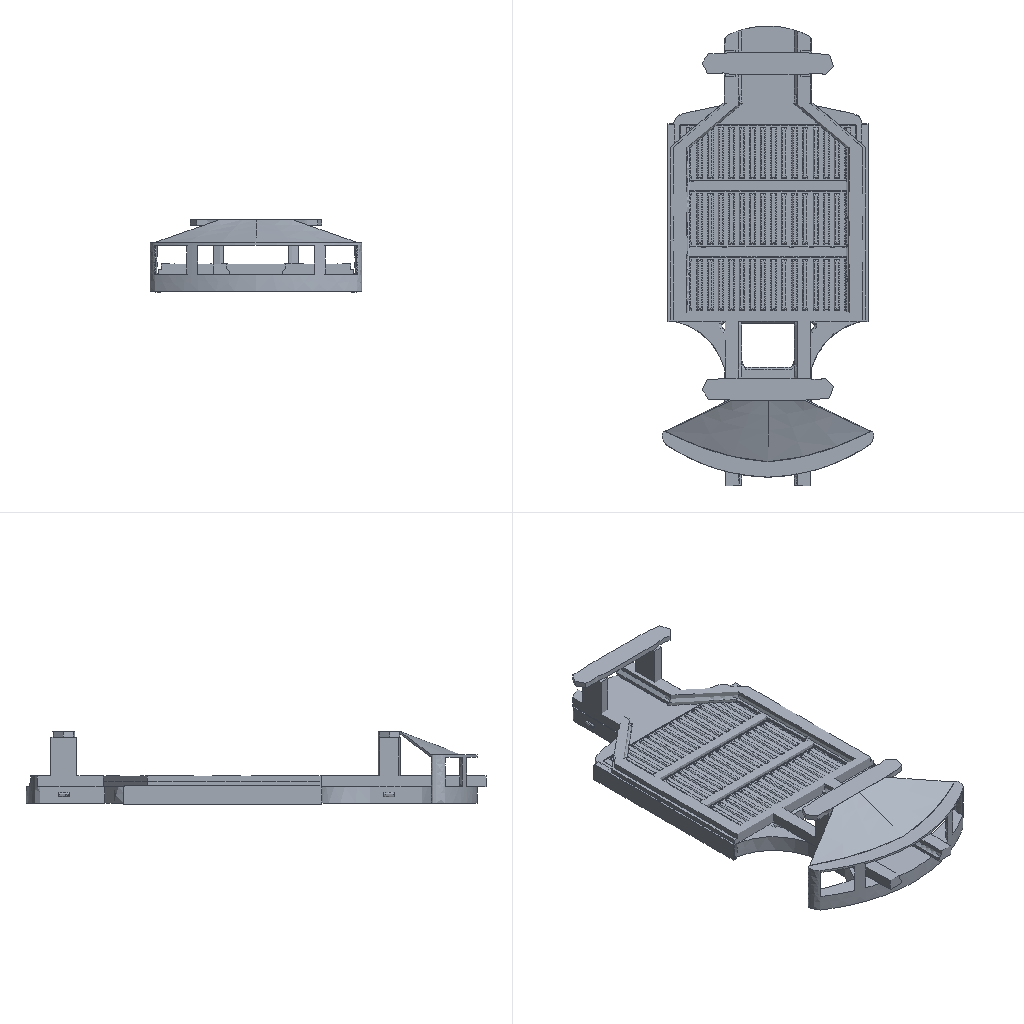Simulation study | ansys workbench
Ansys APDL input file, long lists of numbers shortened:
/batch
/config,noeldb,1     ! force off writing results to database
*get,_wallstrt,active,,time,wall
! ANSYS input file written by Workbench version 2022 R1
! File used for geometry attach: F:\ansys（分析文件汇总)\底盘有限元分析\ansys\dipan.STEP
/title,wbnew--____ (C5)
! ****** Begin Custom Load Command Snippet ******
/COM, ACT Extensions:
/COM,     LSDYNA, 2021.1
/COM,
! ****** End   Custom Load Command Snippet ******
*DIM,_wb_ProjectScratch_dir,string,248
_wb_ProjectScratch_dir(1) = 'C:\Users\Administrator\AppData\Local\Temp\WB_Administrator_26060_2\_ProjectScratch\Scr306D\'
*DIM,_wb_SolverFiles_dir,string,248
_wb_SolverFiles_dir(1) = 'C:\Users\Administrator\AppData\Local\Temp\WB_Administrator_26060_2\wbnew_files\dp0\SYS-1\MECH\'
*DIM,_wb_userfiles_dir,string,248
_wb_userfiles_dir(1) = 'C:\Users\Administrator\AppData\Local\Temp\WB_Administrator_26060_2\wbnew_files\user_files\'
/com,--- Data in consistent NMM units. See Solving Units in the help system for more information.
/units,MPA
/nopr
/wb,file,start              !  signify a WB generated input file
/prep7
! Turn off shape checking because checks already performed inside WB mesher.
! See help system for more information.
SHPP,OFF,,NOWARN
/nolist
etcon,set             ! allow ANSYS to choose best KEYOP's for 180x elements, resets any applicable keyopt to MAPDL defaults
/com,*********** Nodes for the whole assembly ***********
nblock,3,,302792
(1i9,3e20.9e3)
        1     2.552000817E+02    -4.340854422E+02     3.633624358E+02
! (275265 more lines like these left out)
-1
/wb,elem,start            !  set before creation of elements
/com,*********** Elements for Body 1 "dipan-FreeParts|NONE" ***********
et,1,187
eblock,19,solid,,173485
(19i9)
        1        1        1        1        0        0        0        0       10        0       19    13623    39379    40222    40211   140088   275016   140091   140090
! (346969 more lines like these left out)
-1
/com,*********** Elements for Body 2 "dipan-FreeParts|NONE[2]" ***********
et,2,186
keyo,2,2,1          ! set full integration on SOLID186
eblock,19,solid,,9
(19i9)
        2        2        2        2        0        0        0        0       20        0        1        4       21       24       25        5       19       20       16
! (17 more lines like these left out)
-1
/com,*********** Elements for Body 3 "dipan-FreeParts|NONE[3]" ***********
et,3,186
keyo,3,2,1          ! set full integration on SOLID186
eblock,19,solid,,9
(19i9)
        3        3        3        3        0        0        0        0       20        0       10      100      117      120      121      101      115      116      112
! (17 more lines like these left out)
-1
/wb,elem,end               !  done creating elements
/com,*********** Send User Defined Coordinate System(s) ***********
csys,0
toffst,273.15,  ! Temperature offset from absolute zero
/com,*********** Set Reference Temperature ***********
tref,22.
/wb,mat,start              !  starting to send materials
/com,*********** Send Materials ***********
Temperature = 'TEMP' ! Temperature
MP,DENS,1,7.85e-09,	! tonne mm^-3
MP,ALPX,1,1.2e-05,	! C^-1
MP,C,1,434000000,	! mm^2 s^-2 C^-1
MP,KXX,1,60.5,	! tonne mm s^-3 C^-1
MP,RSVX,1,0.00017,	! ohm mm
MP,EX,1,200000,	! tonne s^-2 mm^-1
MP,NUXY,1,0.3,
MP,MURX,1,10000,
Temperature = 'TEMP' ! Temperature
MP,DENS,2,7.85e-09,	! tonne mm^-3
MP,ALPX,2,1.2e-05,	! C^-1
MP,C,2,434000000,	! mm^2 s^-2 C^-1
MP,KXX,2,60.5,	! tonne mm s^-3 C^-1
MP,RSVX,2,0.00017,	! ohm mm
MP,EX,2,200000,	! tonne s^-2 mm^-1
MP,NUXY,2,0.3,
MP,MURX,2,10000,
Temperature = 'TEMP' ! Temperature
MP,DENS,3,7.85e-09,	! tonne mm^-3
MP,ALPX,3,1.2e-05,	! C^-1
MP,C,3,434000000,	! mm^2 s^-2 C^-1
MP,KXX,3,60.5,	! tonne mm s^-3 C^-1
MP,RSVX,3,0.00017,	! ohm mm
MP,EX,3,200000,	! tonne s^-2 mm^-1
MP,NUXY,3,0.3,
MP,MURX,3,10000,
/wb,mat,end                !  done sending materials
!************************* Model Summary ********************
!dipan-FreeParts|NONE,	结构钢,	matid,	1
!dipan-FreeParts|NONE[2],	结构钢,	matid,	2
!dipan-FreeParts|NONE[3],	结构钢,	matid,	3
!************************* End Model Summary ********************
! get the diagonal of the bounding box. Needed later for other things
*get,_xmin,node,,mnloc,x
*get,_ymin,node,,mnloc,y
*get,_zmin,node,,mnloc,z
*get,_xmax,node,,mxloc,x
*get,_ymax,node,,mxloc,y
*get,_zmax,node,,mxloc,z
_ASMDIAG=(_xmax-_xmin)*(_xmax-_xmin)+(_ymax-_ymin)*(_ymax-_ymin)+(_zmax-_zmin)*(_zmax-_zmin)
_ASMDIAG=SQRT(_ASMDIAG)
/wb,contact,start          !  starting to send contact
/com,*********** Create Contact "接触区域 3" ***********
/com,            Real Constant Set For Above Contact Is 5 & 4
*set,tid,5
*set,cid,4
r,tid
r,cid
et,tid,170
et,cid,174
eblock,10,,,3
(15i9)
   216164        5        5        5        0       30       29       12       11       94       69       66       67
   216165        5        5        5        0       29       28       13       12       93       71       68       69
   216166        5        5        5        0       28       23       17       13       88       79       70       71
-1
eblock,10,,,3
(15i9)
   216167        4        4        4        0       30       29       12       11       94       69       66       67
   216168        4        4        4        0       29       28       13       12       93       71       68       69
   216169        4        4        4        0       28       23       17       13       88       79       70       71
-1
eblock,10,,,3
(15i9)
   216170        4        5        4        0      110      111      122      123      168      171      187      169
   216171        4        5        4        0      111      112      121      122      170      173      186      171
   216172        4        5        4        0      112      116      120      121      172      180      185      173
-1
eblock,10,,,3
(15i9)
   216173        5        4        5        0      110      111      122      123      168      171      187      169
   216174        5        4        5        0      111      112      121      122      170      173      186      171
   216175        5        4        5        0      112      116      120      121      172      180      185      173
-1
keyo,cid,8,2               ! auto create asymmetric contact (from Program Controlled setting)
keyo,cid,10,0              ! adjust contact stiffness each NR iteration (from Program Controlled setting)
keyo,cid,12,5              ! bonded always
keyo,cid,18,1              ! small sliding turned on by application
keyo,cid,2,0               ! augmented Lagrange (from Program Controlled setting)
keyo,cid,4,0               ! on Gauss point (from Program Controlled setting)
keyo,cid,9,1               ! ignore initial gaps/penetration
keyo,cid,7,0               ! No Prediction
rmod,tid,3,10.      ! FKN
rmod,tid,5,0.       ! ICONT
rmod,tid,6,0.       ! PINB
rmod,tid,10,0.      ! CNOF
rmod,tid,12,0.      ! FKT
rmod,tid,36,47      ! WB DSID
rmod,cid,3,10.      ! FKN
rmod,cid,5,0.       ! ICONT
rmod,cid,6,0.       ! PINB
rmod,cid,10,0.      ! CNOF
rmod,cid,12,0.      ! FKT
rmod,cid,36,47      ! WB DSID
nsel,all
esel,all
/wb,contact,end            !  done creating contacts
/golist
/wb,load,start             !  starting to send loads
/com,*********** Fixed Supports ***********
CMBLOCK,_FIXEDSU,NODE,      435
(8i10)
         5         6         7         8         9        10        11        12
! (54 more lines like these left out)
cmsel,s,_FIXEDSU
d,all,all
nsel,all
/com,*********** Define Force Using Surface Effect Elements ***********
local,12,0,0.,0.,0.,0.,0.,0.
csys,0
et,6,154
eblock,10,,,13183
(15i9)
   216176        6        6        6       12    13326    13856    13958    13958   137814   141428    13958   137816
! (13182 more lines like these left out)
-1
esel,s,type,,6
keyop,6,2,1                ! Apply load in local coordinate system
keyop,6,7,1                ! Use original area so load is constant in large deformation
esel,all
/gst,on,on
fini
*get,_numnode,node,0,count
*get,_numelem,elem,0,count
*get, _MAXELEMNUM, elem, 0, NUM, MAX
*get, _MAXNODENUM, node, 0, NUM, MAX
*get, _MAXELEMTYPE, etyp, 0, NUM, MAX
*get, _MAXREALCONST, real, 0, NUM, MAX
/go
/wb,load,end               !  done creating loads
/com,--- Number of total nodes = %_numnode%
/com,--- Number of contact elements = 13195
/com,--- Number of spring elements = 0
/com,--- Number of bearing elements = 0
/com,--- Number of solid elements = 173503
/com,--- Number of condensed parts = 0
/com,--- Number of total elements = %_numelem%
*get,_wallbsol,active,,time,wall
/com,****************************************************************************
/com,*************************    SOLUTION       ********************************
/com,****************************************************************************
/solu
antype,0                   ! static analysis
_thickRatio=0.333   ! Ratio of thick parts in the model
eqsl,sparse,,,,,1
cntr,print,1               ! print out contact info and also make no initial contact an error
dmpoption,emat,no             ! Don't combine emat file for DANSYS
dmpoption,esav,no             ! Don't combine esav file for DANSYS
nldiag,cont,iter           ! print out contact info each equilibrium iteration
rescontrol,,none                 ! Do not keep any restart files
/com,****************************************************
/com,******************* SOLVE FOR LS 1 OF 1 ****************
esel,s,type,,6
nsle
sfe,all,1,pres,1,0.
sfe,all,2,pres,1,0.
sfe,all,3,pres,1,-0.1317
nsel,all
esel,all
/nopr
/gopr
nsub,1,1,1
time,1.
outres,erase
outres,all,none
outres,nsol,all,
outres,rsol,all
outres,eangl,all
outres,etmp,all
outres,veng,all
outres,strs,all,
outres,epel,all,
outres,eppl,all,
outres,cont,all,
! *********** WB SOLVE COMMAND ***********
! check interactive state
*get,ANSINTER_,active,,int
*if,ANSINTER_,ne,0,then
/eof
*endif
solve
/com *************** Write FE CONNECTORS *********
CEWRITE,file,ce,,INTE
/com,****************************************************
/com,*************** FINISHED SOLVE FOR LS 1 *************
*get,_wallasol,active,,time,wall
/nopr
*get,_numnode,node,0,count
*get,_numelem,elem,0,count
*get, _MAXELEMNUM, elem, 0, NUM, MAX
*get, _MAXNODENUM, node, 0, NUM, MAX,,,INTERNAL
*get, _MAXELEMTYPE, etyp, 0, NUM, MAX
*get, _MAXREALCONST, real, 0, NUM, MAX
/gopr
/post1
xmlo,ENCODING,ISO-8859-1
xmlo,parm
/xml,parm,xml
fini
/gopr
*get,_walldone,active,,time,wall
_preptime=(_wallbsol-_wallstrt)*3600
_solvtime=(_wallasol-_wallbsol)*3600
_posttime=(_walldone-_wallasol)*3600
_totaltim=(_walldone-_wallstrt)*3600
*get,_dlbratio,active,0,solu,dlbr
*get,_combtime,active,0,solu,comb
*get,_ssmode,active,0,solu,ssmm
*get,_ndofs,active,0,solu,ndof
*get,_sol_end_time,active,0,set,time
*if,_sol_end_time,eq,1.,then
/fclean				!clean distributed files
*endif
/com,--- Total number of nodes = %_numnode%
/com,--- Total number of elements = %_numelem%
/com,--- Element load balance ratio = %_dlbratio%
/com,--- Time to combine distributed files = %_combtime%
/com,--- Sparse memory mode = %_ssmode%
/com,--- Number of DOF = %_ndofs%
/wb,file,end               ! done with WB generated input